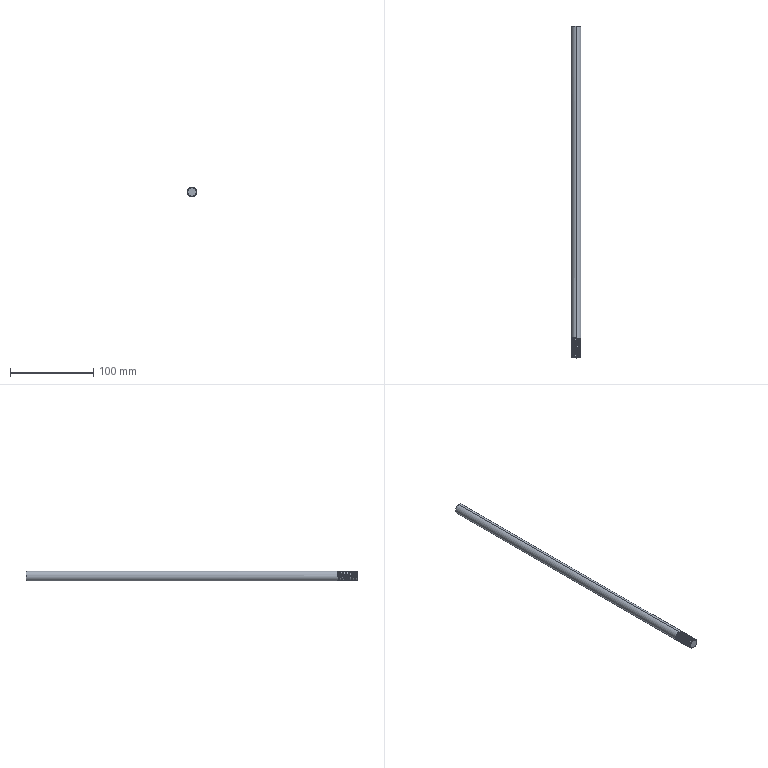Part | SolidWorks | features BaseBody 1 | 1 solid | 62 faces | box 12 x 398.65 x 12 mm | volume 44666 mm3 | cylinder 54 | plane 4 | cone 2 | spline 2 | commonest cylinder face diameters 10.25 x27 12 x27